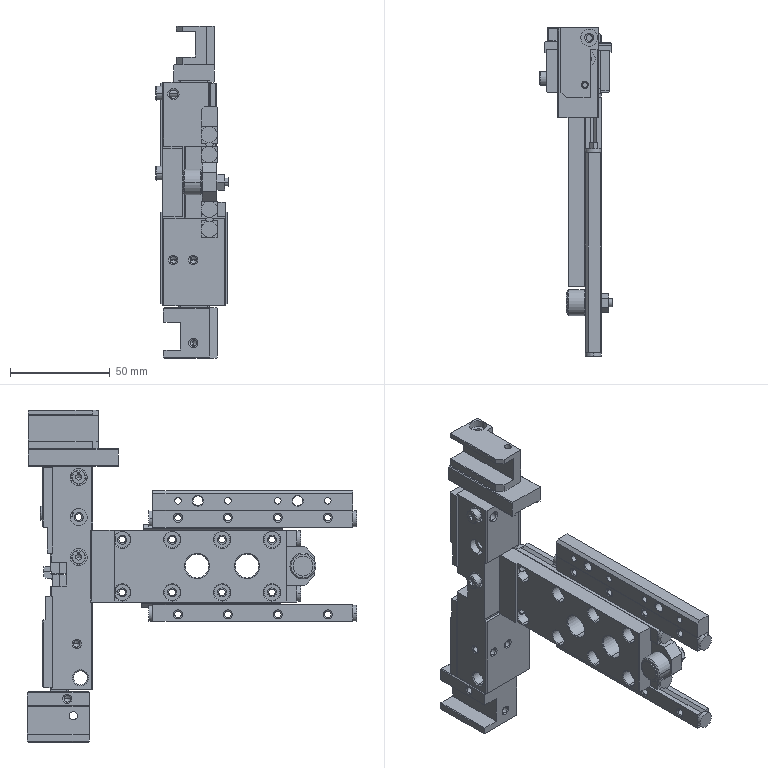Part | NX | 24 solids | 1075 faces | box 36.3 x 164.9 x 166.238 mm | volume 167479 mm3 | plane 511 | cylinder 322 | cone 242 | commonest cylinder face diameters 3.3 x78 6 x44 8 x40 4.5 x32 5 x24 3 x14